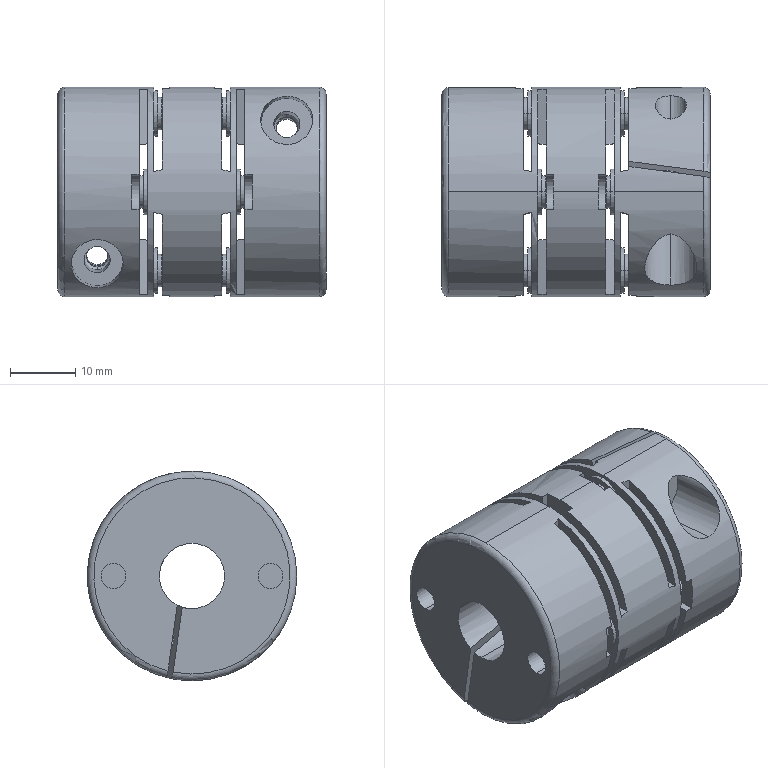Part | SolidWorks | features BaseBody 1 | 1 solid | 174 faces | box 41 x 32 x 32 mm | volume 23223 mm3 | cylinder 89 | plane 75 | cone 8 | torus 2 | commonest cylinder face diameters 5 x16 7 x16 3.8 x8 5.4 x8 16 x8 3.242 x7